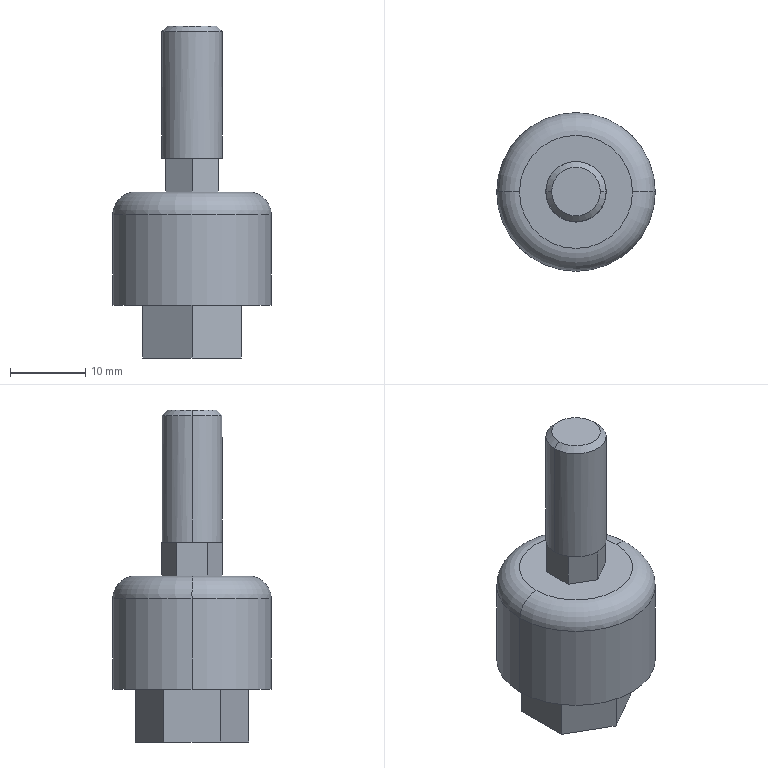Part | STEP file | JA20-8-125 | 1 solid | 41 faces | box 21 x 21 x 44 mm | volume 6882 mm3 | plane 29 | cylinder 6 | cone 4 | torus 2 | commonest cylinder face diameters 6.647 x2 8 x2 21 x2
STEP:
#1=CARTESIAN_POINT('',(-10.5,0.,19.));
#2=VERTEX_POINT('',#1);
#3=CARTESIAN_POINT('',(10.5,0.,19.));
#4=VERTEX_POINT('',#3);
#5=CARTESIAN_POINT('',(0.,0.,19.));
#6=DIRECTION('',(0.,0.,-1.));
#7=DIRECTION('',(1.,0.,0.));
#8=AXIS2_PLACEMENT_3D('',#5,#6,#7);
#9=CIRCLE('',#8,10.5);
#10=EDGE_CURVE('',#2,#4,#9,.T.);
#11=ORIENTED_EDGE('',*,*,#10,.F.);
#12=CARTESIAN_POINT('',(-7.5,0.,22.));
#13=VERTEX_POINT('',#12);
#14=CARTESIAN_POINT('',(-7.5,0.,19.));
#15=DIRECTION('',(0.,1.,0.));
#16=DIRECTION('',(-1.,0.,0.));
#17=AXIS2_PLACEMENT_3D('',#14,#15,#16);
#18=CIRCLE('',#17,3.);
#19=EDGE_CURVE('',#2,#13,#18,.T.);
#20=ORIENTED_EDGE('',*,*,#19,.T.);
#21=CARTESIAN_POINT('',(7.5,0.,22.));
#22=VERTEX_POINT('',#21);
#23=CARTESIAN_POINT('',(0.,0.,22.));
#24=DIRECTION('',(0.,0.,1.));
#25=DIRECTION('',(1.,0.,0.));
#26=AXIS2_PLACEMENT_3D('',#23,#24,#25);
#27=CIRCLE('',#26,7.5);
#28=EDGE_CURVE('',#22,#13,#27,.T.);
#29=ORIENTED_EDGE('',*,*,#28,.F.);
#30=CARTESIAN_POINT('',(7.5,0.,19.));
#31=DIRECTION('',(0.,-1.,0.));
#32=DIRECTION('',(0.,0.,-1.));
#33=AXIS2_PLACEMENT_3D('',#30,#31,#32);
#34=CIRCLE('',#33,3.);
#35=EDGE_CURVE('',#4,#22,#34,.T.);
#36=ORIENTED_EDGE('',*,*,#35,.F.);
#37=EDGE_LOOP('',(#11,#20,#29,#36));
#38=FACE_OUTER_BOUND('',#37,.T.);
#39=CARTESIAN_POINT('',(0.,0.,19.));
#40=DIRECTION('',(0.,0.,1.));
#41=DIRECTION('',(1.,0.,0.));
#42=AXIS2_PLACEMENT_3D('',#39,#40,#41);
#43=TOROIDAL_SURFACE('',#42,7.5,3.);
#44=ADVANCED_FACE('',(#38),#43,.T.);
#45=ORIENTED_EDGE('',*,*,#10,.T.);
#46=CARTESIAN_POINT('',(10.5,0.,7.));
#47=VERTEX_POINT('',#46);
#48=CARTESIAN_POINT('',(10.5,0.,14.5));
#49=DIRECTION('',(0.,0.,-1.));
#50=VECTOR('',#49,1000.);
#51=LINE('',#48,#50);
#52=EDGE_CURVE('',#4,#47,#51,.T.);
#53=ORIENTED_EDGE('',*,*,#52,.T.);
#54=CARTESIAN_POINT('',(-10.5,0.,7.));
#55=VERTEX_POINT('',#54);
#56=CARTESIAN_POINT('',(0.,0.,7.));
#57=DIRECTION('',(0.,0.,1.));
#58=DIRECTION('',(-1.,0.,0.));
#59=AXIS2_PLACEMENT_3D('',#56,#57,#58);
#60=CIRCLE('',#59,10.5);
#61=EDGE_CURVE('',#47,#55,#60,.T.);
#62=ORIENTED_EDGE('',*,*,#61,.T.);
#63=CARTESIAN_POINT('',(-10.5,0.,14.5));
#64=DIRECTION('',(0.,0.,-1.));
#65=VECTOR('',#64,1000.);
#66=LINE('',#63,#65);
#67=EDGE_CURVE('',#2,#55,#66,.T.);
#68=ORIENTED_EDGE('',*,*,#67,.F.);
#69=EDGE_LOOP('',(#45,#53,#62,#68));
#70=FACE_OUTER_BOUND('',#69,.T.);
#71=CARTESIAN_POINT('',(0.,0.,14.5));
#72=DIRECTION('',(0.,0.,-1.));
#73=DIRECTION('',(-1.,0.,0.));
#74=AXIS2_PLACEMENT_3D('',#71,#72,#73);
#75=CYLINDRICAL_SURFACE('',#74,10.5);
#76=ADVANCED_FACE('',(#70),#75,.T.);
#77=CARTESIAN_POINT('',(-4.,0.,43.233));
#78=VERTEX_POINT('',#77);
#79=CARTESIAN_POINT('',(4.,0.,43.233));
#80=VERTEX_POINT('',#79);
#81=CARTESIAN_POINT('',(0.,0.,43.233));
#82=DIRECTION('',(0.,0.,-1.));
#83=DIRECTION('',(-1.,0.,0.));
#84=AXIS2_PLACEMENT_3D('',#81,#82,#83);
#85=CIRCLE('',#84,4.);
#86=EDGE_CURVE('',#78,#80,#85,.T.);
#87=ORIENTED_EDGE('',*,*,#86,.T.);
#88=CARTESIAN_POINT('',(4.,0.,26.5));
#89=VERTEX_POINT('',#88);
#90=CARTESIAN_POINT('',(4.,0.,34.867));
#91=DIRECTION('',(0.,0.,-1.));
#92=VECTOR('',#91,1000.);
#93=LINE('',#90,#92);
#94=EDGE_CURVE('',#80,#89,#93,.T.);
#95=ORIENTED_EDGE('',*,*,#94,.T.);
#96=CARTESIAN_POINT('',(3.5,1.936,26.5));
#97=VERTEX_POINT('',#96);
#98=CARTESIAN_POINT('',(0.,0.,26.5));
#99=DIRECTION('',(0.,0.,-1.));
#100=DIRECTION('',(-1.,0.,0.));
#101=AXIS2_PLACEMENT_3D('',#98,#99,#100);
#102=CIRCLE('',#101,4.);
#103=EDGE_CURVE('',#97,#89,#102,.T.);
#104=ORIENTED_EDGE('',*,*,#103,.F.);
#105=CARTESIAN_POINT('',(3.427,2.063,26.5));
#106=VERTEX_POINT('',#105);
#107=CARTESIAN_POINT('',(0.,0.,26.5));
#108=DIRECTION('',(0.,0.,-1.));
#109=DIRECTION('',(1.,0.,0.));
#110=AXIS2_PLACEMENT_3D('',#107,#108,#109);
#111=CIRCLE('',#110,4.);
#112=EDGE_CURVE('',#106,#97,#111,.T.);
#113=ORIENTED_EDGE('',*,*,#112,.F.);
#114=CARTESIAN_POINT('',(0.07295,3.999,26.5));
#115=VERTEX_POINT('',#114);
#116=CARTESIAN_POINT('',(0.,0.,26.5));
#117=DIRECTION('',(0.,0.,-1.));
#118=DIRECTION('',(-1.,0.,0.));
#119=AXIS2_PLACEMENT_3D('',#116,#117,#118);
#120=CIRCLE('',#119,4.);
#121=EDGE_CURVE('',#115,#106,#120,.T.);
#122=ORIENTED_EDGE('',*,*,#121,.F.);
#123=CARTESIAN_POINT('',(-0.07295,3.999,26.5));
#124=VERTEX_POINT('',#123);
#125=CARTESIAN_POINT('',(0.,0.,26.5));
#126=DIRECTION('',(0.,0.,-1.));
#127=DIRECTION('',(1.,0.,0.));
#128=AXIS2_PLACEMENT_3D('',#125,#126,#127);
#129=CIRCLE('',#128,4.);
#130=EDGE_CURVE('',#124,#115,#129,.T.);
#131=ORIENTED_EDGE('',*,*,#130,.F.);
#132=CARTESIAN_POINT('',(-3.427,2.063,26.5));
#133=VERTEX_POINT('',#132);
#134=CARTESIAN_POINT('',(0.,0.,26.5));
#135=DIRECTION('',(0.,0.,-1.));
#136=DIRECTION('',(-1.,0.,0.));
#137=AXIS2_PLACEMENT_3D('',#134,#135,#136);
#138=CIRCLE('',#137,4.);
#139=EDGE_CURVE('',#133,#124,#138,.T.);
#140=ORIENTED_EDGE('',*,*,#139,.F.);
#141=CARTESIAN_POINT('',(-3.5,1.936,26.5));
#142=VERTEX_POINT('',#141);
#143=CARTESIAN_POINT('',(0.,0.,26.5));
#144=DIRECTION('',(0.,0.,-1.));
#145=DIRECTION('',(1.,0.,0.));
#146=AXIS2_PLACEMENT_3D('',#143,#144,#145);
#147=CIRCLE('',#146,4.);
#148=EDGE_CURVE('',#142,#133,#147,.T.);
#149=ORIENTED_EDGE('',*,*,#148,.F.);
#150=CARTESIAN_POINT('',(-4.,0.,26.5));
#151=VERTEX_POINT('',#150);
#152=CARTESIAN_POINT('',(0.,0.,26.5));
#153=DIRECTION('',(0.,0.,-1.));
#154=DIRECTION('',(-1.,0.,0.));
#155=AXIS2_PLACEMENT_3D('',#152,#153,#154);
#156=CIRCLE('',#155,4.);
#157=EDGE_CURVE('',#151,#142,#156,.T.);
#158=ORIENTED_EDGE('',*,*,#157,.F.);
#159=CARTESIAN_POINT('',(-4.,0.,34.867));
#160=DIRECTION('',(0.,0.,-1.));
#161=VECTOR('',#160,1000.);
#162=LINE('',#159,#161);
#163=EDGE_CURVE('',#78,#151,#162,.T.);
#164=ORIENTED_EDGE('',*,*,#163,.F.);
#165=EDGE_LOOP('',(#87,#95,#104,#113,#122,#131,#140,#149,#158,#164));
#166=FACE_OUTER_BOUND('',#165,.T.);
#167=CARTESIAN_POINT('',(0.,0.,34.867));
#168=DIRECTION('',(0.,0.,-1.));
#169=DIRECTION('',(-1.,0.,0.));
#170=AXIS2_PLACEMENT_3D('',#167,#168,#169);
#171=CYLINDRICAL_SURFACE('',#170,4.);
#172=ADVANCED_FACE('',(#166),#171,.T.);
#173=CARTESIAN_POINT('',(3.324,0.,0.6765));
#174=VERTEX_POINT('',#173);
#175=CARTESIAN_POINT('',(-3.324,0.,0.6765));
#176=VERTEX_POINT('',#175);
#177=CARTESIAN_POINT('',(0.,0.,0.6765));
#178=DIRECTION('',(0.,0.,-1.));
#179=DIRECTION('',(0.,1.,0.));
#180=AXIS2_PLACEMENT_3D('',#177,#178,#179);
#181=CIRCLE('',#180,3.324);
#182=EDGE_CURVE('',#174,#176,#181,.T.);
#183=ORIENTED_EDGE('',*,*,#182,.F.);
#184=CARTESIAN_POINT('',(4.,0.,0.));
#185=VERTEX_POINT('',#184);
#186=CARTESIAN_POINT('',(4.,0.,0.));
#187=DIRECTION('',(0.7071,0.,-0.7071));
#188=VECTOR('',#187,1000.);
#189=LINE('',#186,#188);
#190=EDGE_CURVE('',#174,#185,#189,.T.);
#191=ORIENTED_EDGE('',*,*,#190,.T.);
#192=CARTESIAN_POINT('',(-4.,0.,0.));
#193=VERTEX_POINT('',#192);
#194=CARTESIAN_POINT('',(0.,0.,0.));
#195=DIRECTION('',(0.,0.,1.));
#196=DIRECTION('',(-1.,0.,0.));
#197=AXIS2_PLACEMENT_3D('',#194,#195,#196);
#198=CIRCLE('',#197,4.);
#199=EDGE_CURVE('',#193,#185,#198,.T.);
#200=ORIENTED_EDGE('',*,*,#199,.F.);
#201=CARTESIAN_POINT('',(-4.,0.,0.));
#202=DIRECTION('',(-0.7071,0.,-0.7071));
#203=VECTOR('',#202,1000.);
#204=LINE('',#201,#203);
#205=EDGE_CURVE('',#176,#193,#204,.T.);
#206=ORIENTED_EDGE('',*,*,#205,.F.);
#207=EDGE_LOOP('',(#183,#191,#200,#206));
#208=FACE_OUTER_BOUND('',#207,.T.);
#209=CARTESIAN_POINT('',(0.,0.,0.));
#210=DIRECTION('',(0.,0.,-1.));
#211=DIRECTION('',(-1.,0.,0.));
#212=AXIS2_PLACEMENT_3D('',#209,#210,#211);
#213=CONICAL_SURFACE('',#212,4.,0.7854);
#214=ADVANCED_FACE('',(#208),#213,.F.);
#215=CARTESIAN_POINT('',(-3.233,0.,44.));
#216=VERTEX_POINT('',#215);
#217=CARTESIAN_POINT('',(3.233,0.,44.));
#218=VERTEX_POINT('',#217);
#219=CARTESIAN_POINT('',(0.,0.,44.));
#220=DIRECTION('',(0.,0.,-1.));
#221=DIRECTION('',(-1.,0.,0.));
#222=AXIS2_PLACEMENT_3D('',#219,#220,#221);
#223=CIRCLE('',#222,3.233);
#224=EDGE_CURVE('',#216,#218,#223,.T.);
#225=ORIENTED_EDGE('',*,*,#224,.T.);
#226=CARTESIAN_POINT('',(4.,0.,43.233));
#227=DIRECTION('',(0.7071,0.,-0.7071));
#228=VECTOR('',#227,1000.);
#229=LINE('',#226,#228);
#230=EDGE_CURVE('',#218,#80,#229,.T.);
#231=ORIENTED_EDGE('',*,*,#230,.T.);
#232=ORIENTED_EDGE('',*,*,#86,.F.);
#233=CARTESIAN_POINT('',(-4.,0.,43.233));
#234=DIRECTION('',(-0.7071,0.,-0.7071));
#235=VECTOR('',#234,1000.);
#236=LINE('',#233,#235);
#237=EDGE_CURVE('',#216,#78,#236,.T.);
#238=ORIENTED_EDGE('',*,*,#237,.F.);
#239=EDGE_LOOP('',(#225,#231,#232,#238));
#240=FACE_OUTER_BOUND('',#239,.T.);
#241=CARTESIAN_POINT('',(0.,0.,43.233));
#242=DIRECTION('',(0.,0.,-1.));
#243=DIRECTION('',(-1.,0.,0.));
#244=AXIS2_PLACEMENT_3D('',#241,#242,#243);
#245=CONICAL_SURFACE('',#244,4.,0.7854);
#246=ADVANCED_FACE('',(#240),#245,.T.);
#247=CARTESIAN_POINT('',(3.324,0.,8.));
#248=VERTEX_POINT('',#247);
#249=CARTESIAN_POINT('',(-3.324,0.,8.));
#250=VERTEX_POINT('',#249);
#251=CARTESIAN_POINT('',(0.,0.,8.));
#252=DIRECTION('',(0.,0.,-1.));
#253=DIRECTION('',(-1.,0.,0.));
#254=AXIS2_PLACEMENT_3D('',#251,#252,#253);
#255=CIRCLE('',#254,3.324);
#256=EDGE_CURVE('',#248,#250,#255,.T.);
#257=ORIENTED_EDGE('',*,*,#256,.F.);
#258=CARTESIAN_POINT('',(3.324,0.,4.338));
#259=DIRECTION('',(0.,0.,-1.));
#260=VECTOR('',#259,1000.);
#261=LINE('',#258,#260);
#262=EDGE_CURVE('',#248,#174,#261,.T.);
#263=ORIENTED_EDGE('',*,*,#262,.T.);
#264=ORIENTED_EDGE('',*,*,#182,.T.);
#265=CARTESIAN_POINT('',(-3.324,0.,4.338));
#266=DIRECTION('',(0.,0.,-1.));
#267=VECTOR('',#266,1000.);
#268=LINE('',#265,#267);
#269=EDGE_CURVE('',#250,#176,#268,.T.);
#270=ORIENTED_EDGE('',*,*,#269,.F.);
#271=EDGE_LOOP('',(#257,#263,#264,#270));
#272=FACE_OUTER_BOUND('',#271,.T.);
#273=CARTESIAN_POINT('',(0.,0.,4.338));
#274=DIRECTION('',(0.,0.,-1.));
#275=DIRECTION('',(-1.,0.,0.));
#276=AXIS2_PLACEMENT_3D('',#273,#274,#275);
#277=CYLINDRICAL_SURFACE('',#276,3.324);
#278=ADVANCED_FACE('',(#272),#277,.F.);
#279=ORIENTED_EDGE('',*,*,#52,.F.);
#280=CARTESIAN_POINT('',(0.,0.,19.));
#281=DIRECTION('',(0.,0.,-1.));
#282=DIRECTION('',(1.,0.,0.));
#283=AXIS2_PLACEMENT_3D('',#280,#281,#282);
#284=CIRCLE('',#283,10.5);
#285=EDGE_CURVE('',#4,#2,#284,.T.);
#286=ORIENTED_EDGE('',*,*,#285,.T.);
#287=ORIENTED_EDGE('',*,*,#67,.T.);
#288=CARTESIAN_POINT('',(0.,0.,7.));
#289=DIRECTION('',(0.,0.,1.));
#290=DIRECTION('',(-1.,0.,0.));
#291=AXIS2_PLACEMENT_3D('',#288,#289,#290);
#292=CIRCLE('',#291,10.5);
#293=EDGE_CURVE('',#55,#47,#292,.T.);
#294=ORIENTED_EDGE('',*,*,#293,.T.);
#295=EDGE_LOOP('',(#279,#286,#287,#294));
#296=FACE_OUTER_BOUND('',#295,.T.);
#297=CARTESIAN_POINT('',(0.,0.,14.5));
#298=DIRECTION('',(0.,0.,-1.));
#299=DIRECTION('',(-1.,0.,0.));
#300=AXIS2_PLACEMENT_3D('',#297,#298,#299);
#301=CYLINDRICAL_SURFACE('',#300,10.5);
#302=ADVANCED_FACE('',(#296),#301,.T.);
#303=ORIENTED_EDGE('',*,*,#28,.T.);
#304=CARTESIAN_POINT('',(0.,0.,22.));
#305=DIRECTION('',(0.,0.,1.));
#306=DIRECTION('',(1.,0.,0.));
#307=AXIS2_PLACEMENT_3D('',#304,#305,#306);
#308=CIRCLE('',#307,7.5);
#309=EDGE_CURVE('',#13,#22,#308,.T.);
#310=ORIENTED_EDGE('',*,*,#309,.T.);
#311=EDGE_LOOP('',(#303,#310));
#312=FACE_OUTER_BOUND('',#311,.T.);
#313=CARTESIAN_POINT('',(3.5,2.021,22.));
#314=VERTEX_POINT('',#313);
#315=CARTESIAN_POINT('',(3.5,-2.021,22.));
#316=VERTEX_POINT('',#315);
#317=CARTESIAN_POINT('',(3.5,5.25,22.));
#318=DIRECTION('',(0.,-1.,0.));
#319=VECTOR('',#318,1000.);
#320=LINE('',#317,#319);
#321=EDGE_CURVE('',#314,#316,#320,.T.);
#322=ORIENTED_EDGE('',*,*,#321,.T.);
#323=CARTESIAN_POINT('',(0.,-4.041,22.));
#324=VERTEX_POINT('',#323);
#325=CARTESIAN_POINT('',(3.5,-2.021,22.));
#326=DIRECTION('',(-0.866,-0.5,0.));
#327=VECTOR('',#326,1000.);
#328=LINE('',#325,#327);
#329=EDGE_CURVE('',#316,#324,#328,.T.);
#330=ORIENTED_EDGE('',*,*,#329,.T.);
#331=CARTESIAN_POINT('',(-3.5,-2.021,22.));
#332=VERTEX_POINT('',#331);
#333=CARTESIAN_POINT('',(0.,-4.041,22.));
#334=DIRECTION('',(-0.866,0.5,0.));
#335=VECTOR('',#334,1000.);
#336=LINE('',#333,#335);
#337=EDGE_CURVE('',#324,#332,#336,.T.);
#338=ORIENTED_EDGE('',*,*,#337,.T.);
#339=CARTESIAN_POINT('',(-3.5,2.021,22.));
#340=VERTEX_POINT('',#339);
#341=CARTESIAN_POINT('',(-3.5,5.25,22.));
#342=DIRECTION('',(0.,1.,0.));
#343=VECTOR('',#342,1000.);
#344=LINE('',#341,#343);
#345=EDGE_CURVE('',#332,#340,#344,.T.);
#346=ORIENTED_EDGE('',*,*,#345,.T.);
#347=CARTESIAN_POINT('',(0.,4.041,22.));
#348=VERTEX_POINT('',#347);
#349=CARTESIAN_POINT('',(-3.5,2.021,22.));
#350=DIRECTION('',(0.866,0.5,0.));
#351=VECTOR('',#350,1000.);
#352=LINE('',#349,#351);
#353=EDGE_CURVE('',#340,#348,#352,.T.);
#354=ORIENTED_EDGE('',*,*,#353,.T.);
#355=CARTESIAN_POINT('',(0.,4.041,22.));
#356=DIRECTION('',(0.866,-0.5,0.));
#357=VECTOR('',#356,1000.);
#358=LINE('',#355,#357);
#359=EDGE_CURVE('',#348,#314,#358,.T.);
#360=ORIENTED_EDGE('',*,*,#359,.T.);
#361=EDGE_LOOP('',(#322,#330,#338,#346,#354,#360));
#362=FACE_BOUND('',#361,.T.);
#363=CARTESIAN_POINT('',(0.,5.25,22.));
#364=DIRECTION('',(0.,0.,1.));
#365=DIRECTION('',(1.,0.,0.));
#366=AXIS2_PLACEMENT_3D('',#363,#364,#365);
#367=PLANE('',#366);
#368=ADVANCED_FACE('',(#312,#362),#367,.T.);
#369=ORIENTED_EDGE('',*,*,#293,.F.);
#370=ORIENTED_EDGE('',*,*,#61,.F.);
#371=EDGE_LOOP('',(#369,#370));
#372=FACE_OUTER_BOUND('',#371,.T.);
#373=CARTESIAN_POINT('',(6.5,3.753,7.));
#374=VERTEX_POINT('',#373);
#375=CARTESIAN_POINT('',(0.,7.506,7.));
#376=VERTEX_POINT('',#375);
#377=CARTESIAN_POINT('',(6.5,3.753,7.));
#378=DIRECTION('',(-0.866,0.5,0.));
#379=VECTOR('',#378,1000.);
#380=LINE('',#377,#379);
#381=EDGE_CURVE('',#374,#376,#380,.T.);
#382=ORIENTED_EDGE('',*,*,#381,.T.);
#383=CARTESIAN_POINT('',(-6.5,3.753,7.));
#384=VERTEX_POINT('',#383);
#385=CARTESIAN_POINT('',(0.,7.506,7.));
#386=DIRECTION('',(-0.866,-0.5,0.));
#387=VECTOR('',#386,1000.);
#388=LINE('',#385,#387);
#389=EDGE_CURVE('',#376,#384,#388,.T.);
#390=ORIENTED_EDGE('',*,*,#389,.T.);
#391=CARTESIAN_POINT('',(-6.5,-3.753,7.));
#392=VERTEX_POINT('',#391);
#393=CARTESIAN_POINT('',(-6.5,9.15,7.));
#394=DIRECTION('',(0.,-1.,0.));
#395=VECTOR('',#394,1000.);
#396=LINE('',#393,#395);
#397=EDGE_CURVE('',#384,#392,#396,.T.);
#398=ORIENTED_EDGE('',*,*,#397,.T.);
#399=CARTESIAN_POINT('',(0.,-7.506,7.));
#400=VERTEX_POINT('',#399);
#401=CARTESIAN_POINT('',(-6.5,-3.753,7.));
#402=DIRECTION('',(0.866,-0.5,0.));
#403=VECTOR('',#402,1000.);
#404=LINE('',#401,#403);
#405=EDGE_CURVE('',#392,#400,#404,.T.);
#406=ORIENTED_EDGE('',*,*,#405,.T.);
#407=CARTESIAN_POINT('',(6.5,-3.753,7.));
#408=VERTEX_POINT('',#407);
#409=CARTESIAN_POINT('',(0.,-7.506,7.));
#410=DIRECTION('',(0.866,0.5,0.));
#411=VECTOR('',#410,1000.);
#412=LINE('',#409,#411);
#413=EDGE_CURVE('',#400,#408,#412,.T.);
#414=ORIENTED_EDGE('',*,*,#413,.T.);
#415=CARTESIAN_POINT('',(6.5,9.15,7.));
#416=DIRECTION('',(0.,1.,0.));
#417=VECTOR('',#416,1000.);
#418=LINE('',#415,#417);
#419=EDGE_CURVE('',#408,#374,#418,.T.);
#420=ORIENTED_EDGE('',*,*,#419,.T.);
#421=EDGE_LOOP('',(#382,#390,#398,#406,#414,#420));
#422=FACE_BOUND('',#421,.T.);
#423=CARTESIAN_POINT('',(0.,9.15,7.));
#424=DIRECTION('',(0.,0.,-1.));
#425=DIRECTION('',(-1.,0.,0.));
#426=AXIS2_PLACEMENT_3D('',#423,#424,#425);
#427=PLANE('',#426);
#428=ADVANCED_FACE('',(#372,#422),#427,.T.);
#429=CARTESIAN_POINT('',(0.07295,-3.999,26.5));
#430=VERTEX_POINT('',#429);
#431=CARTESIAN_POINT('',(0.,-4.041,26.5));
#432=VERTEX_POINT('',#431);
#433=CARTESIAN_POINT('',(0.,-4.041,26.5));
#434=DIRECTION('',(-0.866,-0.5,0.));
#435=VECTOR('',#434,1000.);
#436=LINE('',#433,#435);
#437=EDGE_CURVE('',#430,#432,#436,.T.);
#438=ORIENTED_EDGE('',*,*,#437,.T.);
#439=CARTESIAN_POINT('',(0.,-4.041,26.5));
#440=DIRECTION('',(0.,0.,-1.));
#441=VECTOR('',#440,1000.);
#442=LINE('',#439,#441);
#443=EDGE_CURVE('',#432,#324,#442,.T.);
#444=ORIENTED_EDGE('',*,*,#443,.T.);
#445=ORIENTED_EDGE('',*,*,#329,.F.);
#446=CARTESIAN_POINT('',(3.5,-2.021,26.5));
#447=VERTEX_POINT('',#446);
#448=CARTESIAN_POINT('',(3.5,-2.021,26.5));
#449=DIRECTION('',(0.,0.,1.));
#450=VECTOR('',#449,1000.);
#451=LINE('',#448,#450);
#452=EDGE_CURVE('',#316,#447,#451,.T.);
#453=ORIENTED_EDGE('',*,*,#452,.T.);
#454=CARTESIAN_POINT('',(3.427,-2.063,26.5));
#455=VERTEX_POINT('',#454);
#456=CARTESIAN_POINT('',(0.,-4.041,26.5));
#457=DIRECTION('',(-0.866,-0.5,0.));
#458=VECTOR('',#457,1000.);
#459=LINE('',#456,#458);
#460=EDGE_CURVE('',#447,#455,#459,.T.);
#461=ORIENTED_EDGE('',*,*,#460,.T.);
#462=CARTESIAN_POINT('',(0.,-4.041,26.5));
#463=DIRECTION('',(-0.866,-0.5,0.));
#464=VECTOR('',#463,1000.);
#465=LINE('',#462,#464);
#466=EDGE_CURVE('',#455,#430,#465,.T.);
#467=ORIENTED_EDGE('',*,*,#466,.T.);
#468=EDGE_LOOP('',(#438,#444,#445,#453,#461,#467));
#469=FACE_OUTER_BOUND('',#468,.T.);
#470=CARTESIAN_POINT('',(0.,-4.041,26.5));
#471=DIRECTION('',(0.5,-0.866,0.));
#472=DIRECTION('',(0.866,0.5,0.));
#473=AXIS2_PLACEMENT_3D('',#470,#471,#472);
#474=PLANE('',#473);
#475=ADVANCED_FACE('',(#469),#474,.T.);
#476=CARTESIAN_POINT('',(3.5,-1.936,26.5));
#477=VERTEX_POINT('',#476);
#478=CARTESIAN_POINT('',(3.5,-2.021,26.5));
#479=DIRECTION('',(0.,-1.,0.));
#480=VECTOR('',#479,1000.);
#481=LINE('',#478,#480);
#482=EDGE_CURVE('',#477,#447,#481,.T.);
#483=ORIENTED_EDGE('',*,*,#482,.T.);
#484=ORIENTED_EDGE('',*,*,#452,.F.);
#485=ORIENTED_EDGE('',*,*,#321,.F.);
#486=CARTESIAN_POINT('',(3.5,2.021,26.5));
#487=VERTEX_POINT('',#486);
#488=CARTESIAN_POINT('',(3.5,2.021,26.5));
#489=DIRECTION('',(0.,0.,1.));
#490=VECTOR('',#489,1000.);
#491=LINE('',#488,#490);
#492=EDGE_CURVE('',#314,#487,#491,.T.);
#493=ORIENTED_EDGE('',*,*,#492,.T.);
#494=CARTESIAN_POINT('',(3.5,-2.021,26.5));
#495=DIRECTION('',(0.,-1.,0.));
#496=VECTOR('',#495,1000.);
#497=LINE('',#494,#496);
#498=EDGE_CURVE('',#487,#97,#497,.T.);
#499=ORIENTED_EDGE('',*,*,#498,.T.);
#500=CARTESIAN_POINT('',(3.5,-2.021,26.5));
#501=DIRECTION('',(0.,-1.,0.));
#502=VECTOR('',#501,1000.);
#503=LINE('',#500,#502);
#504=EDGE_CURVE('',#97,#477,#503,.T.);
#505=ORIENTED_EDGE('',*,*,#504,.T.);
#506=EDGE_LOOP('',(#483,#484,#485,#493,#499,#505));
#507=FACE_OUTER_BOUND('',#506,.T.);
#508=CARTESIAN_POINT('',(3.5,-2.021,26.5));
#509=DIRECTION('',(1.,0.,0.));
#510=DIRECTION('',(0.,0.,-1.));
#511=AXIS2_PLACEMENT_3D('',#508,#509,#510);
#512=PLANE('',#511);
#513=ADVANCED_FACE('',(#507),#512,.T.);
#514=CARTESIAN_POINT('',(3.5,2.021,26.5));
#515=DIRECTION('',(0.866,-0.5,0.));
#516=VECTOR('',#515,1000.);
#517=LINE('',#514,#516);
#518=EDGE_CURVE('',#106,#487,#517,.T.);
#519=ORIENTED_EDGE('',*,*,#518,.T.);
#520=ORIENTED_EDGE('',*,*,#492,.F.);
#521=ORIENTED_EDGE('',*,*,#359,.F.);
#522=CARTESIAN_POINT('',(0.,4.041,26.5));
#523=VERTEX_POINT('',#522);
#524=CARTESIAN_POINT('',(0.,4.041,26.5));
#525=DIRECTION('',(0.,0.,1.));
#526=VECTOR('',#525,1000.);
#527=LINE('',#524,#526);
#528=EDGE_CURVE('',#348,#523,#527,.T.);
#529=ORIENTED_EDGE('',*,*,#528,.T.);
#530=CARTESIAN_POINT('',(3.5,2.021,26.5));
#531=DIRECTION('',(0.866,-0.5,0.));
#532=VECTOR('',#531,1000.);
#533=LINE('',#530,#532);
#534=EDGE_CURVE('',#523,#115,#533,.T.);
#535=ORIENTED_EDGE('',*,*,#534,.T.);
#536=CARTESIAN_POINT('',(3.5,2.021,26.5));
#537=DIRECTION('',(0.866,-0.5,0.));
#538=VECTOR('',#537,1000.);
#539=LINE('',#536,#538);
#540=EDGE_CURVE('',#115,#106,#539,.T.);
#541=ORIENTED_EDGE('',*,*,#540,.T.);
#542=EDGE_LOOP('',(#519,#520,#521,#529,#535,#541));
#543=FACE_OUTER_BOUND('',#542,.T.);
#544=CARTESIAN_POINT('',(3.5,2.021,26.5));
#545=DIRECTION('',(0.5,0.866,0.));
#546=DIRECTION('',(-0.866,0.5,0.));
#547=AXIS2_PLACEMENT_3D('',#544,#545,#546);
#548=PLANE('',#547);
#549=ADVANCED_FACE('',(#543),#548,.T.);
#550=CARTESIAN_POINT('',(0.,4.041,26.5));
#551=DIRECTION('',(0.866,0.5,0.));
#552=VECTOR('',#551,1000.);
#553=LINE('',#550,#552);
#554=EDGE_CURVE('',#124,#523,#553,.T.);
#555=ORIENTED_EDGE('',*,*,#554,.T.);
#556=ORIENTED_EDGE('',*,*,#528,.F.);
#557=ORIENTED_EDGE('',*,*,#353,.F.);
#558=CARTESIAN_POINT('',(-3.5,2.021,26.5));
#559=VERTEX_POINT('',#558);
#560=CARTESIAN_POINT('',(-3.5,2.021,26.5));
#561=DIRECTION('',(0.,0.,1.));
#562=VECTOR('',#561,1000.);
#563=LINE('',#560,#562);
#564=EDGE_CURVE('',#340,#559,#563,.T.);
#565=ORIENTED_EDGE('',*,*,#564,.T.);
#566=CARTESIAN_POINT('',(0.,4.041,26.5));
#567=DIRECTION('',(0.866,0.5,0.));
#568=VECTOR('',#567,1000.);
#569=LINE('',#566,#568);
#570=EDGE_CURVE('',#559,#133,#569,.T.);
#571=ORIENTED_EDGE('',*,*,#570,.T.);
#572=CARTESIAN_POINT('',(0.,4.041,26.5));
#573=DIRECTION('',(0.866,0.5,0.));
#574=VECTOR('',#573,1000.);
#575=LINE('',#572,#574);
#576=EDGE_CURVE('',#133,#124,#575,.T.);
#577=ORIENTED_EDGE('',*,*,#576,.T.);
#578=EDGE_LOOP('',(#555,#556,#557,#565,#571,#577));
#579=FACE_OUTER_BOUND('',#578,.T.);
#580=CARTESIAN_POINT('',(0.,4.041,26.5));
#581=DIRECTION('',(-0.5,0.866,0.));
#582=DIRECTION('',(-0.866,-0.5,0.));
#583=AXIS2_PLACEMENT_3D('',#580,#581,#582);
#584=PLANE('',#583);
#585=ADVANCED_FACE('',(#579),#584,.T.);
#586=CARTESIAN_POINT('',(-3.5,2.021,26.5));
#587=DIRECTION('',(0.,1.,0.));
#588=VECTOR('',#587,1000.);
#589=LINE('',#586,#588);
#590=EDGE_CURVE('',#142,#559,#589,.T.);
#591=ORIENTED_EDGE('',*,*,#590,.T.);
#592=ORIENTED_EDGE('',*,*,#564,.F.);
#593=ORIENTED_EDGE('',*,*,#345,.F.);
#594=CARTESIAN_POINT('',(-3.5,-2.021,26.5));
#595=VERTEX_POINT('',#594);
#596=CARTESIAN_POINT('',(-3.5,-2.021,26.5));
#597=DIRECTION('',(0.,0.,1.));
#598=VECTOR('',#597,1000.);
#599=LINE('',#596,#598);
#600=EDGE_CURVE('',#332,#595,#599,.T.);
#601=ORIENTED_EDGE('',*,*,#600,.T.);
#602=CARTESIAN_POINT('',(-3.5,-1.936,26.5));
#603=VERTEX_POINT('',#602);
#604=CARTESIAN_POINT('',(-3.5,2.021,26.5));
#605=DIRECTION('',(0.,1.,0.));
#606=VECTOR('',#605,1000.);
#607=LINE('',#604,#606);
#608=EDGE_CURVE('',#595,#603,#607,.T.);
#609=ORIENTED_EDGE('',*,*,#608,.T.);
#610=CARTESIAN_POINT('',(-3.5,2.021,26.5));
#611=DIRECTION('',(0.,1.,0.));
#612=VECTOR('',#611,1000.);
#613=LINE('',#610,#612);
#614=EDGE_CURVE('',#603,#142,#613,.T.);
#615=ORIENTED_EDGE('',*,*,#614,.T.);
#616=EDGE_LOOP('',(#591,#592,#593,#601,#609,#615));
#617=FACE_OUTER_BOUND('',#616,.T.);
#618=CARTESIAN_POINT('',(-3.5,2.021,26.5));
#619=DIRECTION('',(-1.,0.,0.));
#620=DIRECTION('',(0.,0.,1.));
#621=AXIS2_PLACEMENT_3D('',#618,#619,#620);
#622=PLANE('',#621);
#623=ADVANCED_FACE('',(#617),#622,.T.);
#624=CARTESIAN_POINT('',(-3.427,-2.063,26.5));
#625=VERTEX_POINT('',#624);
#626=CARTESIAN_POINT('',(-3.5,-2.021,26.5));
#627=DIRECTION('',(-0.866,0.5,0.));
#628=VECTOR('',#627,1000.);
#629=LINE('',#626,#628);
#630=EDGE_CURVE('',#625,#595,#629,.T.);
#631=ORIENTED_EDGE('',*,*,#630,.T.);
#632=ORIENTED_EDGE('',*,*,#600,.F.);
#633=ORIENTED_EDGE('',*,*,#337,.F.);
#634=ORIENTED_EDGE('',*,*,#443,.F.);
#635=CARTESIAN_POINT('',(-0.07295,-3.999,26.5));
#636=VERTEX_POINT('',#635);
#637=CARTESIAN_POINT('',(-3.5,-2.021,26.5));
#638=DIRECTION('',(-0.866,0.5,0.));
#639=VECTOR('',#638,1000.);
#640=LINE('',#637,#639);
#641=EDGE_CURVE('',#432,#636,#640,.T.);
#642=ORIENTED_EDGE('',*,*,#641,.T.);
#643=CARTESIAN_POINT('',(-3.5,-2.021,26.5));
#644=DIRECTION('',(-0.866,0.5,0.));
#645=VECTOR('',#644,1000.);
#646=LINE('',#643,#645);
#647=EDGE_CURVE('',#636,#625,#646,.T.);
#648=ORIENTED_EDGE('',*,*,#647,.T.);
#649=EDGE_LOOP('',(#631,#632,#633,#634,#642,#648));
#650=FACE_OUTER_BOUND('',#649,.T.);
#651=CARTESIAN_POINT('',(-3.5,-2.021,26.5));
#652=DIRECTION('',(-0.5,-0.866,0.));
#653=DIRECTION('',(0.866,-0.5,0.));
#654=AXIS2_PLACEMENT_3D('',#651,#652,#653);
#655=PLANE('',#654);
#656=ADVANCED_FACE('',(#650),#655,.T.);
#657=CARTESIAN_POINT('',(0.,7.506,0.));
#658=VERTEX_POINT('',#657);
#659=CARTESIAN_POINT('',(0.,7.506,0.));
#660=DIRECTION('',(0.,0.,1.));
#661=VECTOR('',#660,1000.);
#662=LINE('',#659,#661);
#663=EDGE_CURVE('',#658,#376,#662,.T.);
#664=ORIENTED_EDGE('',*,*,#663,.F.);
#665=CARTESIAN_POINT('',(-6.5,3.753,0.));
#666=VERTEX_POINT('',#665);
#667=CARTESIAN_POINT('',(0.,7.506,0.));
#668=DIRECTION('',(0.866,0.5,0.));
#669=VECTOR('',#668,1000.);
#670=LINE('',#667,#669);
#671=EDGE_CURVE('',#666,#658,#670,.T.);
#672=ORIENTED_EDGE('',*,*,#671,.F.);
#673=CARTESIAN_POINT('',(-6.5,3.753,0.));
#674=DIRECTION('',(0.,0.,-1.));
#675=VECTOR('',#674,1000.);
#676=LINE('',#673,#675);
#677=EDGE_CURVE('',#384,#666,#676,.T.);
#678=ORIENTED_EDGE('',*,*,#677,.F.);
#679=ORIENTED_EDGE('',*,*,#389,.F.);
#680=EDGE_LOOP('',(#664,#672,#678,#679));
#681=FACE_OUTER_BOUND('',#680,.T.);
#682=CARTESIAN_POINT('',(0.,7.506,0.));
#683=DIRECTION('',(0.5,-0.866,0.));
#684=DIRECTION('',(0.866,0.5,0.));
#685=AXIS2_PLACEMENT_3D('',#682,#683,#684);
#686=PLANE('',#685);
#687=ADVANCED_FACE('',(#681),#686,.F.);
#688=CARTESIAN_POINT('',(6.5,3.753,0.));
#689=VERTEX_POINT('',#688);
#690=CARTESIAN_POINT('',(6.5,3.753,0.));
#691=DIRECTION('',(0.,0.,1.));
#692=VECTOR('',#691,1000.);
#693=LINE('',#690,#692);
#694=EDGE_CURVE('',#689,#374,#693,.T.);
#695=ORIENTED_EDGE('',*,*,#694,.F.);
#696=CARTESIAN_POINT('',(6.5,3.753,0.));
#697=DIRECTION('',(0.866,-0.5,0.));
#698=VECTOR('',#697,1000.);
#699=LINE('',#696,#698);
#700=EDGE_CURVE('',#658,#689,#699,.T.);
#701=ORIENTED_EDGE('',*,*,#700,.F.);
#702=ORIENTED_EDGE('',*,*,#663,.T.);
#703=ORIENTED_EDGE('',*,*,#381,.F.);
#704=EDGE_LOOP('',(#695,#701,#702,#703));
#705=FACE_OUTER_BOUND('',#704,.T.);
#706=CARTESIAN_POINT('',(6.5,3.753,0.));
#707=DIRECTION('',(-0.5,-0.866,0.));
#708=DIRECTION('',(0.866,-0.5,0.));
#709=AXIS2_PLACEMENT_3D('',#706,#707,#708);
#710=PLANE('',#709);
#711=ADVANCED_FACE('',(#705),#710,.F.);
#712=CARTESIAN_POINT('',(6.5,-3.753,0.));
#713=VERTEX_POINT('',#712);
#714=CARTESIAN_POINT('',(6.5,-3.753,0.));
#715=DIRECTION('',(0.,0.,1.));
#716=VECTOR('',#715,1000.);
#717=LINE('',#714,#716);
#718=EDGE_CURVE('',#713,#408,#717,.T.);
#719=ORIENTED_EDGE('',*,*,#718,.F.);
#720=CARTESIAN_POINT('',(6.5,-3.753,0.));
#721=DIRECTION('',(0.,-1.,0.));
#722=VECTOR('',#721,1000.);
#723=LINE('',#720,#722);
#724=EDGE_CURVE('',#689,#713,#723,.T.);
#725=ORIENTED_EDGE('',*,*,#724,.F.);
#726=ORIENTED_EDGE('',*,*,#694,.T.);
#727=ORIENTED_EDGE('',*,*,#419,.F.);
#728=EDGE_LOOP('',(#719,#725,#726,#727));
#729=FACE_OUTER_BOUND('',#728,.T.);
#730=CARTESIAN_POINT('',(6.5,-3.753,0.));
#731=DIRECTION('',(-1.,0.,0.));
#732=DIRECTION('',(0.,0.,1.));
#733=AXIS2_PLACEMENT_3D('',#730,#731,#732);
#734=PLANE('',#733);
#735=ADVANCED_FACE('',(#729),#734,.F.);
#736=CARTESIAN_POINT('',(0.,-7.506,0.));
#737=VERTEX_POINT('',#736);
#738=CARTESIAN_POINT('',(0.,-7.506,0.));
#739=DIRECTION('',(0.,0.,1.));
#740=VECTOR('',#739,1000.);
#741=LINE('',#738,#740);
#742=EDGE_CURVE('',#737,#400,#741,.T.);
#743=ORIENTED_EDGE('',*,*,#742,.F.);
#744=CARTESIAN_POINT('',(0.,-7.506,0.));
#745=DIRECTION('',(-0.866,-0.5,0.));
#746=VECTOR('',#745,1000.);
#747=LINE('',#744,#746);
#748=EDGE_CURVE('',#713,#737,#747,.T.);
#749=ORIENTED_EDGE('',*,*,#748,.F.);
#750=ORIENTED_EDGE('',*,*,#718,.T.);
#751=ORIENTED_EDGE('',*,*,#413,.F.);
#752=EDGE_LOOP('',(#743,#749,#750,#751));
#753=FACE_OUTER_BOUND('',#752,.T.);
#754=CARTESIAN_POINT('',(0.,-7.506,0.));
#755=DIRECTION('',(-0.5,0.866,0.));
#756=DIRECTION('',(-0.866,-0.5,0.));
#757=AXIS2_PLACEMENT_3D('',#754,#755,#756);
#758=PLANE('',#757);
#759=ADVANCED_FACE('',(#753),#758,.F.);
#760=CARTESIAN_POINT('',(-6.5,-3.753,0.));
#761=VERTEX_POINT('',#760);
#762=CARTESIAN_POINT('',(-6.5,-3.753,0.));
#763=DIRECTION('',(0.,0.,1.));
#764=VECTOR('',#763,1000.);
#765=LINE('',#762,#764);
#766=EDGE_CURVE('',#761,#392,#765,.T.);
#767=ORIENTED_EDGE('',*,*,#766,.F.);
#768=CARTESIAN_POINT('',(-6.5,-3.753,0.));
#769=DIRECTION('',(-0.866,0.5,0.));
#770=VECTOR('',#769,1000.);
#771=LINE('',#768,#770);
#772=EDGE_CURVE('',#737,#761,#771,.T.);
#773=ORIENTED_EDGE('',*,*,#772,.F.);
#774=ORIENTED_EDGE('',*,*,#742,.T.);
#775=ORIENTED_EDGE('',*,*,#405,.F.);
#776=EDGE_LOOP('',(#767,#773,#774,#775));
#777=FACE_OUTER_BOUND('',#776,.T.);
#778=CARTESIAN_POINT('',(-6.5,-3.753,0.));
#779=DIRECTION('',(0.5,0.866,0.));
#780=DIRECTION('',(-0.866,0.5,0.));
#781=AXIS2_PLACEMENT_3D('',#778,#779,#780);
#782=PLANE('',#781);
#783=ADVANCED_FACE('',(#777),#782,.F.);
#784=ORIENTED_EDGE('',*,*,#677,.T.);
#785=CARTESIAN_POINT('',(-6.5,3.753,0.));
#786=DIRECTION('',(0.,1.,0.));
#787=VECTOR('',#786,1000.);
#788=LINE('',#785,#787);
#789=EDGE_CURVE('',#761,#666,#788,.T.);
#790=ORIENTED_EDGE('',*,*,#789,.F.);
#791=ORIENTED_EDGE('',*,*,#766,.T.);
#792=ORIENTED_EDGE('',*,*,#397,.F.);
#793=EDGE_LOOP('',(#784,#790,#791,#792));
#794=FACE_OUTER_BOUND('',#793,.T.);
#795=CARTESIAN_POINT('',(-6.5,3.753,0.));
#796=DIRECTION('',(1.,0.,0.));
#797=DIRECTION('',(0.,0.,-1.));
#798=AXIS2_PLACEMENT_3D('',#795,#796,#797);
#799=PLANE('',#798);
#800=ADVANCED_FACE('',(#794),#799,.F.);
#801=ORIENTED_EDGE('',*,*,#641,.F.);
#802=ORIENTED_EDGE('',*,*,#437,.F.);
#803=CARTESIAN_POINT('',(0.,0.,26.5));
#804=DIRECTION('',(0.,0.,1.));
#805=DIRECTION('',(-1.,0.,0.));
#806=AXIS2_PLACEMENT_3D('',#803,#804,#805);
#807=CIRCLE('',#806,4.);
#808=EDGE_CURVE('',#636,#430,#807,.T.);
#809=ORIENTED_EDGE('',*,*,#808,.F.);
#810=EDGE_LOOP('',(#801,#802,#809));
#811=FACE_OUTER_BOUND('',#810,.T.);
#812=CARTESIAN_POINT('',(0.,0.,26.5));
#813=DIRECTION('',(0.,0.,1.));
#814=DIRECTION('',(1.,0.,0.));
#815=AXIS2_PLACEMENT_3D('',#812,#813,#814);
#816=PLANE('',#815);
#817=ADVANCED_FACE('',(#811),#816,.T.);
#818=ORIENTED_EDGE('',*,*,#466,.F.);
#819=CARTESIAN_POINT('',(0.,0.,26.5));
#820=DIRECTION('',(0.,0.,-1.));
#821=DIRECTION('',(-1.,0.,0.));
#822=AXIS2_PLACEMENT_3D('',#819,#820,#821);
#823=CIRCLE('',#822,4.);
#824=EDGE_CURVE('',#455,#430,#823,.T.);
#825=ORIENTED_EDGE('',*,*,#824,.T.);
#826=EDGE_LOOP('',(#818,#825));
#827=FACE_OUTER_BOUND('',#826,.T.);
#828=CARTESIAN_POINT('',(0.,2.,26.5));
#829=DIRECTION('',(0.,0.,-1.));
#830=DIRECTION('',(-1.,0.,0.));
#831=AXIS2_PLACEMENT_3D('',#828,#829,#830);
#832=PLANE('',#831);
#833=ADVANCED_FACE('',(#827),#832,.T.);
#834=ORIENTED_EDGE('',*,*,#460,.F.);
#835=ORIENTED_EDGE('',*,*,#482,.F.);
#836=CARTESIAN_POINT('',(0.,0.,26.5));
#837=DIRECTION('',(0.,0.,-1.));
#838=DIRECTION('',(1.,0.,0.));
#839=AXIS2_PLACEMENT_3D('',#836,#837,#838);
#840=CIRCLE('',#839,4.);
#841=EDGE_CURVE('',#477,#455,#840,.T.);
#842=ORIENTED_EDGE('',*,*,#841,.T.);
#843=EDGE_LOOP('',(#834,#835,#842));
#844=FACE_OUTER_BOUND('',#843,.T.);
#845=CARTESIAN_POINT('',(0.,0.,26.5));
#846=DIRECTION('',(0.,0.,1.));
#847=DIRECTION('',(1.,0.,0.));
#848=AXIS2_PLACEMENT_3D('',#845,#846,#847);
#849=PLANE('',#848);
#850=ADVANCED_FACE('',(#844),#849,.T.);
#851=ORIENTED_EDGE('',*,*,#504,.F.);
#852=ORIENTED_EDGE('',*,*,#103,.T.);
#853=CARTESIAN_POINT('',(0.,0.,26.5));
#854=DIRECTION('',(0.,0.,-1.));
#855=DIRECTION('',(-1.,0.,0.));
#856=AXIS2_PLACEMENT_3D('',#853,#854,#855);
#857=CIRCLE('',#856,4.);
#858=EDGE_CURVE('',#89,#477,#857,.T.);
#859=ORIENTED_EDGE('',*,*,#858,.T.);
#860=EDGE_LOOP('',(#851,#852,#859));
#861=FACE_OUTER_BOUND('',#860,.T.);
#862=CARTESIAN_POINT('',(0.,2.,26.5));
#863=DIRECTION('',(0.,0.,-1.));
#864=DIRECTION('',(-1.,0.,0.));
#865=AXIS2_PLACEMENT_3D('',#862,#863,#864);
#866=PLANE('',#865);
#867=ADVANCED_FACE('',(#861),#866,.T.);
#868=ORIENTED_EDGE('',*,*,#498,.F.);
#869=ORIENTED_EDGE('',*,*,#518,.F.);
#870=ORIENTED_EDGE('',*,*,#112,.T.);
#871=EDGE_LOOP('',(#868,#869,#870));
#872=FACE_OUTER_BOUND('',#871,.T.);
#873=CARTESIAN_POINT('',(0.,0.,26.5));
#874=DIRECTION('',(0.,0.,1.));
#875=DIRECTION('',(1.,0.,0.));
#876=AXIS2_PLACEMENT_3D('',#873,#874,#875);
#877=PLANE('',#876);
#878=ADVANCED_FACE('',(#872),#877,.T.);
#879=ORIENTED_EDGE('',*,*,#540,.F.);
#880=ORIENTED_EDGE('',*,*,#121,.T.);
#881=EDGE_LOOP('',(#879,#880));
#882=FACE_OUTER_BOUND('',#881,.T.);
#883=CARTESIAN_POINT('',(0.,2.,26.5));
#884=DIRECTION('',(0.,0.,-1.));
#885=DIRECTION('',(-1.,0.,0.));
#886=AXIS2_PLACEMENT_3D('',#883,#884,#885);
#887=PLANE('',#886);
#888=ADVANCED_FACE('',(#882),#887,.T.);
#889=ORIENTED_EDGE('',*,*,#534,.F.);
#890=ORIENTED_EDGE('',*,*,#554,.F.);
#891=ORIENTED_EDGE('',*,*,#130,.T.);
#892=EDGE_LOOP('',(#889,#890,#891));
#893=FACE_OUTER_BOUND('',#892,.T.);
#894=CARTESIAN_POINT('',(0.,0.,26.5));
#895=DIRECTION('',(0.,0.,1.));
#896=DIRECTION('',(1.,0.,0.));
#897=AXIS2_PLACEMENT_3D('',#894,#895,#896);
#898=PLANE('',#897);
#899=ADVANCED_FACE('',(#893),#898,.T.);
#900=ORIENTED_EDGE('',*,*,#576,.F.);
#901=ORIENTED_EDGE('',*,*,#139,.T.);
#902=EDGE_LOOP('',(#900,#901));
#903=FACE_OUTER_BOUND('',#902,.T.);
#904=CARTESIAN_POINT('',(0.,2.,26.5));
#905=DIRECTION('',(0.,0.,-1.));
#906=DIRECTION('',(-1.,0.,0.));
#907=AXIS2_PLACEMENT_3D('',#904,#905,#906);
#908=PLANE('',#907);
#909=ADVANCED_FACE('',(#903),#908,.T.);
#910=ORIENTED_EDGE('',*,*,#570,.F.);
#911=ORIENTED_EDGE('',*,*,#590,.F.);
#912=ORIENTED_EDGE('',*,*,#148,.T.);
#913=EDGE_LOOP('',(#910,#911,#912));
#914=FACE_OUTER_BOUND('',#913,.T.);
#915=CARTESIAN_POINT('',(0.,0.,26.5));
#916=DIRECTION('',(0.,0.,1.));
#917=DIRECTION('',(1.,0.,0.));
#918=AXIS2_PLACEMENT_3D('',#915,#916,#917);
#919=PLANE('',#918);
#920=ADVANCED_FACE('',(#914),#919,.T.);
#921=ORIENTED_EDGE('',*,*,#614,.F.);
#922=CARTESIAN_POINT('',(0.,0.,26.5));
#923=DIRECTION('',(0.,0.,-1.));
#924=DIRECTION('',(-1.,0.,0.));
#925=AXIS2_PLACEMENT_3D('',#922,#923,#924);
#926=CIRCLE('',#925,4.);
#927=EDGE_CURVE('',#603,#151,#926,.T.);
#928=ORIENTED_EDGE('',*,*,#927,.T.);
#929=ORIENTED_EDGE('',*,*,#157,.T.);
#930=EDGE_LOOP('',(#921,#928,#929));
#931=FACE_OUTER_BOUND('',#930,.T.);
#932=CARTESIAN_POINT('',(0.,2.,26.5));
#933=DIRECTION('',(0.,0.,-1.));
#934=DIRECTION('',(-1.,0.,0.));
#935=AXIS2_PLACEMENT_3D('',#932,#933,#934);
#936=PLANE('',#935);
#937=ADVANCED_FACE('',(#931),#936,.T.);
#938=ORIENTED_EDGE('',*,*,#608,.F.);
#939=ORIENTED_EDGE('',*,*,#630,.F.);
#940=CARTESIAN_POINT('',(0.,0.,26.5));
#941=DIRECTION('',(0.,0.,-1.));
#942=DIRECTION('',(1.,0.,0.));
#943=AXIS2_PLACEMENT_3D('',#940,#941,#942);
#944=CIRCLE('',#943,4.);
#945=EDGE_CURVE('',#625,#603,#944,.T.);
#946=ORIENTED_EDGE('',*,*,#945,.T.);
#947=EDGE_LOOP('',(#938,#939,#946));
#948=FACE_OUTER_BOUND('',#947,.T.);
#949=CARTESIAN_POINT('',(0.,0.,26.5));
#950=DIRECTION('',(0.,0.,1.));
#951=DIRECTION('',(1.,0.,0.));
#952=AXIS2_PLACEMENT_3D('',#949,#950,#951);
#953=PLANE('',#952);
#954=ADVANCED_FACE('',(#948),#953,.T.);
#955=ORIENTED_EDGE('',*,*,#647,.F.);
#956=CARTESIAN_POINT('',(0.,0.,26.5));
#957=DIRECTION('',(0.,0.,-1.));
#958=DIRECTION('',(-1.,0.,0.));
#959=AXIS2_PLACEMENT_3D('',#956,#957,#958);
#960=CIRCLE('',#959,4.);
#961=EDGE_CURVE('',#636,#625,#960,.T.);
#962=ORIENTED_EDGE('',*,*,#961,.T.);
#963=EDGE_LOOP('',(#955,#962));
#964=FACE_OUTER_BOUND('',#963,.T.);
#965=CARTESIAN_POINT('',(0.,2.,26.5));
#966=DIRECTION('',(0.,0.,-1.));
#967=DIRECTION('',(-1.,0.,0.));
#968=AXIS2_PLACEMENT_3D('',#965,#966,#967);
#969=PLANE('',#968);
#970=ADVANCED_FACE('',(#964),#969,.T.);
#971=ORIENTED_EDGE('',*,*,#199,.T.);
#972=CARTESIAN_POINT('',(0.,0.,0.));
#973=DIRECTION('',(0.,0.,1.));
#974=DIRECTION('',(-1.,0.,0.));
#975=AXIS2_PLACEMENT_3D('',#972,#973,#974);
#976=CIRCLE('',#975,4.);
#977=EDGE_CURVE('',#185,#193,#976,.T.);
#978=ORIENTED_EDGE('',*,*,#977,.T.);
#979=EDGE_LOOP('',(#971,#978));
#980=FACE_BOUND('',#979,.T.);
#981=ORIENTED_EDGE('',*,*,#748,.T.);
#982=ORIENTED_EDGE('',*,*,#772,.T.);
#983=ORIENTED_EDGE('',*,*,#789,.T.);
#984=ORIENTED_EDGE('',*,*,#671,.T.);
#985=ORIENTED_EDGE('',*,*,#700,.T.);
#986=ORIENTED_EDGE('',*,*,#724,.T.);
#987=EDGE_LOOP('',(#981,#982,#983,#984,#985,#986));
#988=FACE_OUTER_BOUND('',#987,.T.);
#989=CARTESIAN_POINT('',(0.,5.9,0.));
#990=DIRECTION('',(0.,0.,-1.));
#991=DIRECTION('',(-1.,0.,0.));
#992=AXIS2_PLACEMENT_3D('',#989,#990,#991);
#993=PLANE('',#992);
#994=ADVANCED_FACE('',(#980,#988),#993,.T.);
#995=ORIENTED_EDGE('',*,*,#94,.F.);
#996=CARTESIAN_POINT('',(0.,0.,43.233));
#997=DIRECTION('',(0.,0.,-1.));
#998=DIRECTION('',(-1.,0.,0.));
#999=AXIS2_PLACEMENT_3D('',#996,#997,#998);
#1000=CIRCLE('',#999,4.);
#1001=EDGE_CURVE('',#80,#78,#1000,.T.);
#1002=ORIENTED_EDGE('',*,*,#1001,.T.);
#1003=ORIENTED_EDGE('',*,*,#163,.T.);
#1004=ORIENTED_EDGE('',*,*,#927,.F.);
#1005=ORIENTED_EDGE('',*,*,#945,.F.);
#1006=ORIENTED_EDGE('',*,*,#961,.F.);
#1007=ORIENTED_EDGE('',*,*,#808,.T.);
#1008=ORIENTED_EDGE('',*,*,#824,.F.);
#1009=ORIENTED_EDGE('',*,*,#841,.F.);
#1010=ORIENTED_EDGE('',*,*,#858,.F.);
#1011=EDGE_LOOP('',(#995,#1002,#1003,#1004,#1005,#1006,#1007,#1008,#1009,#1010));
#1012=FACE_OUTER_BOUND('',#1011,.T.);
#1013=CARTESIAN_POINT('',(0.,0.,34.867));
#1014=DIRECTION('',(0.,0.,-1.));
#1015=DIRECTION('',(-1.,0.,0.));
#1016=AXIS2_PLACEMENT_3D('',#1013,#1014,#1015);
#1017=CYLINDRICAL_SURFACE('',#1016,4.);
#1018=ADVANCED_FACE('',(#1012),#1017,.T.);
#1019=ORIENTED_EDGE('',*,*,#190,.F.);
#1020=CARTESIAN_POINT('',(0.,0.,0.6765));
#1021=DIRECTION('',(0.,0.,-1.));
#1022=DIRECTION('',(0.,1.,0.));
#1023=AXIS2_PLACEMENT_3D('',#1020,#1021,#1022);
#1024=CIRCLE('',#1023,3.324);
#1025=EDGE_CURVE('',#176,#174,#1024,.T.);
#1026=ORIENTED_EDGE('',*,*,#1025,.F.);
#1027=ORIENTED_EDGE('',*,*,#205,.T.);
#1028=ORIENTED_EDGE('',*,*,#977,.F.);
#1029=EDGE_LOOP('',(#1019,#1026,#1027,#1028));
#1030=FACE_OUTER_BOUND('',#1029,.T.);
#1031=CARTESIAN_POINT('',(0.,0.,0.));
#1032=DIRECTION('',(0.,0.,-1.));
#1033=DIRECTION('',(-1.,0.,0.));
#1034=AXIS2_PLACEMENT_3D('',#1031,#1032,#1033);
#1035=CONICAL_SURFACE('',#1034,4.,0.7854);
#1036=ADVANCED_FACE('',(#1030),#1035,.F.);
#1037=ORIENTED_EDGE('',*,*,#230,.F.);
#1038=CARTESIAN_POINT('',(0.,0.,44.));
#1039=DIRECTION('',(0.,0.,-1.));
#1040=DIRECTION('',(-1.,0.,0.));
#1041=AXIS2_PLACEMENT_3D('',#1038,#1039,#1040);
#1042=CIRCLE('',#1041,3.233);
#1043=EDGE_CURVE('',#218,#216,#1042,.T.);
#1044=ORIENTED_EDGE('',*,*,#1043,.T.);
#1045=ORIENTED_EDGE('',*,*,#237,.T.);
#1046=ORIENTED_EDGE('',*,*,#1001,.F.);
#1047=EDGE_LOOP('',(#1037,#1044,#1045,#1046));
#1048=FACE_OUTER_BOUND('',#1047,.T.);
#1049=CARTESIAN_POINT('',(0.,0.,43.233));
#1050=DIRECTION('',(0.,0.,-1.));
#1051=DIRECTION('',(-1.,0.,0.));
#1052=AXIS2_PLACEMENT_3D('',#1049,#1050,#1051);
#1053=CONICAL_SURFACE('',#1052,4.,0.7854);
#1054=ADVANCED_FACE('',(#1048),#1053,.T.);
#1055=ORIENTED_EDGE('',*,*,#262,.F.);
#1056=CARTESIAN_POINT('',(0.,0.,8.));
#1057=DIRECTION('',(0.,0.,-1.));
#1058=DIRECTION('',(-1.,0.,0.));
#1059=AXIS2_PLACEMENT_3D('',#1056,#1057,#1058);
#1060=CIRCLE('',#1059,3.324);
#1061=EDGE_CURVE('',#250,#248,#1060,.T.);
#1062=ORIENTED_EDGE('',*,*,#1061,.F.);
#1063=ORIENTED_EDGE('',*,*,#269,.T.);
#1064=ORIENTED_EDGE('',*,*,#1025,.T.);
#1065=EDGE_LOOP('',(#1055,#1062,#1063,#1064));
#1066=FACE_OUTER_BOUND('',#1065,.T.);
#1067=CARTESIAN_POINT('',(0.,0.,4.338));
#1068=DIRECTION('',(0.,0.,-1.));
#1069=DIRECTION('',(-1.,0.,0.));
#1070=AXIS2_PLACEMENT_3D('',#1067,#1068,#1069);
#1071=CYLINDRICAL_SURFACE('',#1070,3.324);
#1072=ADVANCED_FACE('',(#1066),#1071,.F.);
#1073=ORIENTED_EDGE('',*,*,#224,.F.);
#1074=ORIENTED_EDGE('',*,*,#1043,.F.);
#1075=EDGE_LOOP('',(#1073,#1074));
#1076=FACE_OUTER_BOUND('',#1075,.T.);
#1077=CARTESIAN_POINT('',(0.,1.617,44.));
#1078=DIRECTION('',(0.,0.,1.));
#1079=DIRECTION('',(1.,0.,0.));
#1080=AXIS2_PLACEMENT_3D('',#1077,#1078,#1079);
#1081=PLANE('',#1080);
#1082=ADVANCED_FACE('',(#1076),#1081,.T.);
#1083=ORIENTED_EDGE('',*,*,#1061,.T.);
#1084=ORIENTED_EDGE('',*,*,#256,.T.);
#1085=EDGE_LOOP('',(#1083,#1084));
#1086=FACE_OUTER_BOUND('',#1085,.T.);
#1087=CARTESIAN_POINT('',(0.,1.662,8.));
#1088=DIRECTION('',(0.,0.,-1.));
#1089=DIRECTION('',(-1.,0.,0.));
#1090=AXIS2_PLACEMENT_3D('',#1087,#1088,#1089);
#1091=PLANE('',#1090);
#1092=ADVANCED_FACE('',(#1086),#1091,.T.);
#1093=ORIENTED_EDGE('',*,*,#19,.F.);
#1094=ORIENTED_EDGE('',*,*,#285,.F.);
#1095=ORIENTED_EDGE('',*,*,#35,.T.);
#1096=ORIENTED_EDGE('',*,*,#309,.F.);
#1097=EDGE_LOOP('',(#1093,#1094,#1095,#1096));
#1098=FACE_OUTER_BOUND('',#1097,.T.);
#1099=CARTESIAN_POINT('',(0.,0.,19.));
#1100=DIRECTION('',(0.,0.,1.));
#1101=DIRECTION('',(1.,0.,0.));
#1102=AXIS2_PLACEMENT_3D('',#1099,#1100,#1101);
#1103=TOROIDAL_SURFACE('',#1102,7.5,3.);
#1104=ADVANCED_FACE('',(#1098),#1103,.T.);
#1105=CLOSED_SHELL('',(#44,#76,#172,#214,#246,#278,#302,#368,#428,#475,#513,#549,#585,#623,#656,#687,#711,#735,#759,#783,#800,#817,#833,#850,#867,#878,#888,#899,#909,#920,#937,#954,#970,#994,#1018,#1036,#1054,#1072,#1082,#1092,#1104));
#1106=MANIFOLD_SOLID_BREP('',#1105);
#1107=CARTESIAN_POINT('',(0.,0.,0.));
#1108=DIRECTION('',(0.,0.,1.));
#1109=DIRECTION('',(1.,0.,0.));
#1110=AXIS2_PLACEMENT_3D('',#1107,#1108,#1109);
#1111=(LENGTH_UNIT()NAMED_UNIT(*)SI_UNIT(.MILLI.,.METRE.));
#1112=UNCERTAINTY_MEASURE_WITH_UNIT(LENGTH_MEASURE(0.00001),#1111,'','');
#1113=(NAMED_UNIT(*)PLANE_ANGLE_UNIT()SI_UNIT($,.RADIAN.));
#1114=(NAMED_UNIT(*)SI_UNIT($,.STERADIAN.)SOLID_ANGLE_UNIT());
#1115=(GEOMETRIC_REPRESENTATION_CONTEXT(3)GLOBAL_UNCERTAINTY_ASSIGNED_CONTEXT((#1112))GLOBAL_UNIT_ASSIGNED_CONTEXT((#1111,#1113,#1114))REPRESENTATION_CONTEXT('',''));
#1116=ADVANCED_BREP_SHAPE_REPRESENTATION('',(#1106,#1110),#1115);